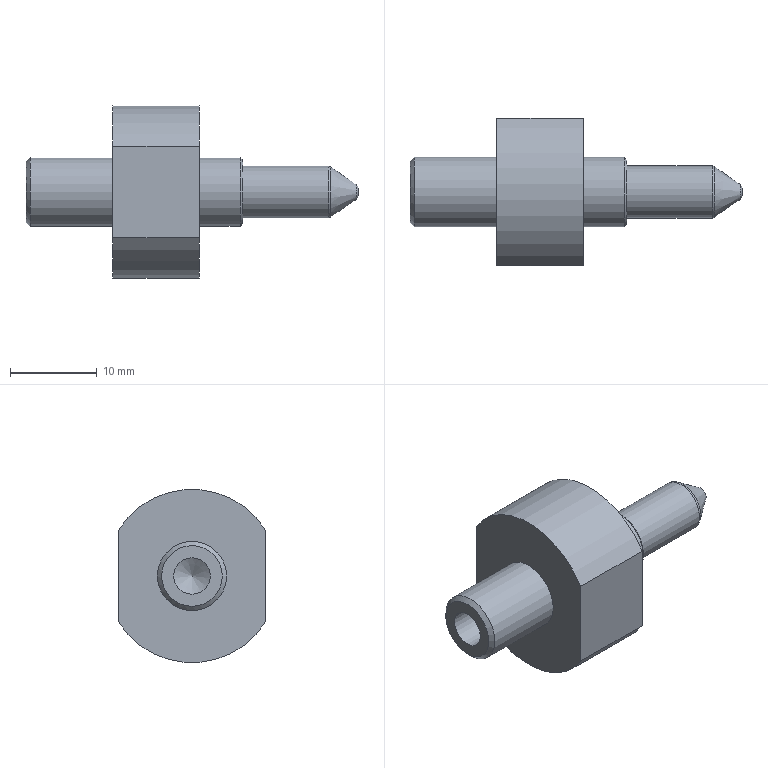Part | NX | features BREP 1 | 1 solid | 19 faces | box 38.285 x 17 x 20 mm | volume 3822 mm3 | plane 7 | cylinder 6 | cone 4 | torus 2 | commonest cylinder face diameters 8 x2 20 x2 4.2 x1 6 x1
STEP:
#1=CARTESIAN_POINT('',(-9.142,8.5,-5.268));
#2=VERTEX_POINT('',#1);
#3=CARTESIAN_POINT('',(-9.142,8.5,5.268));
#4=VERTEX_POINT('',#3);
#5=CARTESIAN_POINT('',(-9.142,8.5,0.));
#6=DIRECTION('',(0.,0.,1.));
#7=VECTOR('',#6,1000.);
#8=LINE('',#5,#7);
#9=EDGE_CURVE('',#2,#4,#8,.T.);
#10=ORIENTED_EDGE('',*,*,#9,.F.);
#11=CARTESIAN_POINT('',(-9.142,-8.5,-5.268));
#12=VERTEX_POINT('',#11);
#13=CARTESIAN_POINT('',(-9.142,0.,0.));
#14=DIRECTION('',(1.,0.,0.));
#15=DIRECTION('',(0.,-1.,0.));
#16=AXIS2_PLACEMENT_3D('',#13,#14,#15);
#17=CIRCLE('',#16,10.);
#18=EDGE_CURVE('',#12,#2,#17,.T.);
#19=ORIENTED_EDGE('',*,*,#18,.F.);
#20=CARTESIAN_POINT('',(-9.142,-8.5,5.268));
#21=VERTEX_POINT('',#20);
#22=CARTESIAN_POINT('',(-9.142,-8.5,0.));
#23=DIRECTION('',(0.,0.,-1.));
#24=VECTOR('',#23,1000.);
#25=LINE('',#22,#24);
#26=EDGE_CURVE('',#21,#12,#25,.T.);
#27=ORIENTED_EDGE('',*,*,#26,.F.);
#28=CARTESIAN_POINT('',(-9.142,0.,0.));
#29=DIRECTION('',(1.,0.,0.));
#30=DIRECTION('',(0.,-1.,0.));
#31=AXIS2_PLACEMENT_3D('',#28,#29,#30);
#32=CIRCLE('',#31,10.);
#33=EDGE_CURVE('',#4,#21,#32,.T.);
#34=ORIENTED_EDGE('',*,*,#33,.F.);
#35=EDGE_LOOP('',(#10,#19,#27,#34));
#36=FACE_BOUND('',#35,.T.);
#37=CARTESIAN_POINT('',(-9.142,-4.,0.));
#38=VERTEX_POINT('',#37);
#39=CARTESIAN_POINT('',(-9.142,0.,0.));
#40=DIRECTION('',(-1.,0.,0.));
#41=DIRECTION('',(0.,-1.,0.));
#42=AXIS2_PLACEMENT_3D('',#39,#40,#41);
#43=CIRCLE('',#42,4.);
#44=EDGE_CURVE('',#38,#38,#43,.T.);
#45=ORIENTED_EDGE('',*,*,#44,.F.);
#46=EDGE_LOOP('',(#45));
#47=FACE_BOUND('',#46,.T.);
#48=CARTESIAN_POINT('',(-9.142,10.,0.));
#49=DIRECTION('',(1.,0.,0.));
#50=DIRECTION('',(0.,-1.,0.));
#51=AXIS2_PLACEMENT_3D('',#48,#49,#50);
#52=PLANE('',#51);
#53=ADVANCED_FACE('',(#36,#47),#52,.F.);
#54=ORIENTED_EDGE('',*,*,#33,.T.);
#55=CARTESIAN_POINT('',(0.8576,-8.5,5.268));
#56=VERTEX_POINT('',#55);
#57=CARTESIAN_POINT('',(-19.142,-8.5,5.268));
#58=DIRECTION('',(1.,0.,0.));
#59=VECTOR('',#58,1000.);
#60=LINE('',#57,#59);
#61=EDGE_CURVE('',#21,#56,#60,.T.);
#62=ORIENTED_EDGE('',*,*,#61,.T.);
#63=CARTESIAN_POINT('',(0.8576,8.5,5.268));
#64=VERTEX_POINT('',#63);
#65=CARTESIAN_POINT('',(0.8576,0.,0.));
#66=DIRECTION('',(-1.,0.,0.));
#67=DIRECTION('',(0.,-1.,0.));
#68=AXIS2_PLACEMENT_3D('',#65,#66,#67);
#69=CIRCLE('',#68,10.);
#70=EDGE_CURVE('',#56,#64,#69,.T.);
#71=ORIENTED_EDGE('',*,*,#70,.T.);
#72=CARTESIAN_POINT('',(-19.142,8.5,5.268));
#73=DIRECTION('',(-1.,0.,0.));
#74=VECTOR('',#73,1000.);
#75=LINE('',#72,#74);
#76=EDGE_CURVE('',#64,#4,#75,.T.);
#77=ORIENTED_EDGE('',*,*,#76,.T.);
#78=EDGE_LOOP('',(#54,#62,#71,#77));
#79=FACE_BOUND('',#78,.T.);
#80=CARTESIAN_POINT('',(-19.142,0.,0.));
#81=DIRECTION('',(-1.,0.,0.));
#82=DIRECTION('',(0.,1.,0.));
#83=AXIS2_PLACEMENT_3D('',#80,#81,#82);
#84=CYLINDRICAL_SURFACE('',#83,10.);
#85=ADVANCED_FACE('',(#79),#84,.T.);
#86=CARTESIAN_POINT('',(0.8576,8.5,-5.268));
#87=VERTEX_POINT('',#86);
#88=CARTESIAN_POINT('',(19.142,8.5,-5.268));
#89=DIRECTION('',(1.,0.,0.));
#90=VECTOR('',#89,1000.);
#91=LINE('',#88,#90);
#92=EDGE_CURVE('',#2,#87,#91,.T.);
#93=ORIENTED_EDGE('',*,*,#92,.F.);
#94=ORIENTED_EDGE('',*,*,#9,.T.);
#95=ORIENTED_EDGE('',*,*,#76,.F.);
#96=CARTESIAN_POINT('',(0.8576,8.5,15.997));
#97=DIRECTION('',(0.,0.,1.));
#98=VECTOR('',#97,1000.);
#99=LINE('',#96,#98);
#100=EDGE_CURVE('',#87,#64,#99,.T.);
#101=ORIENTED_EDGE('',*,*,#100,.F.);
#102=EDGE_LOOP('',(#93,#94,#95,#101));
#103=FACE_BOUND('',#102,.T.);
#104=CARTESIAN_POINT('',(19.142,8.5,15.997));
#105=DIRECTION('',(0.,-1.,0.));
#106=DIRECTION('',(0.,0.,1.));
#107=AXIS2_PLACEMENT_3D('',#104,#105,#106);
#108=PLANE('',#107);
#109=ADVANCED_FACE('',(#103),#108,.F.);
#110=CARTESIAN_POINT('',(0.8576,-8.5,-5.268));
#111=VERTEX_POINT('',#110);
#112=CARTESIAN_POINT('',(0.8576,0.,0.));
#113=DIRECTION('',(-1.,0.,0.));
#114=DIRECTION('',(0.,-1.,0.));
#115=AXIS2_PLACEMENT_3D('',#112,#113,#114);
#116=CIRCLE('',#115,10.);
#117=EDGE_CURVE('',#87,#111,#116,.T.);
#118=ORIENTED_EDGE('',*,*,#117,.T.);
#119=CARTESIAN_POINT('',(-19.142,-8.5,-5.268));
#120=DIRECTION('',(-1.,0.,0.));
#121=VECTOR('',#120,1000.);
#122=LINE('',#119,#121);
#123=EDGE_CURVE('',#111,#12,#122,.T.);
#124=ORIENTED_EDGE('',*,*,#123,.T.);
#125=ORIENTED_EDGE('',*,*,#18,.T.);
#126=ORIENTED_EDGE('',*,*,#92,.T.);
#127=EDGE_LOOP('',(#118,#124,#125,#126));
#128=FACE_BOUND('',#127,.T.);
#129=CARTESIAN_POINT('',(-19.142,0.,0.));
#130=DIRECTION('',(-1.,0.,0.));
#131=DIRECTION('',(0.,1.,0.));
#132=AXIS2_PLACEMENT_3D('',#129,#130,#131);
#133=CYLINDRICAL_SURFACE('',#132,10.);
#134=ADVANCED_FACE('',(#128),#133,.T.);
#135=ORIENTED_EDGE('',*,*,#61,.F.);
#136=ORIENTED_EDGE('',*,*,#26,.T.);
#137=ORIENTED_EDGE('',*,*,#123,.F.);
#138=CARTESIAN_POINT('',(0.8576,-8.5,13.741));
#139=DIRECTION('',(0.,0.,-1.));
#140=VECTOR('',#139,1000.);
#141=LINE('',#138,#140);
#142=EDGE_CURVE('',#56,#111,#141,.T.);
#143=ORIENTED_EDGE('',*,*,#142,.F.);
#144=EDGE_LOOP('',(#135,#136,#137,#143));
#145=FACE_BOUND('',#144,.T.);
#146=CARTESIAN_POINT('',(19.142,-8.5,13.741));
#147=DIRECTION('',(0.,1.,0.));
#148=DIRECTION('',(0.,0.,-1.));
#149=AXIS2_PLACEMENT_3D('',#146,#147,#148);
#150=PLANE('',#149);
#151=ADVANCED_FACE('',(#145),#150,.F.);
#152=CARTESIAN_POINT('',(-18.642,-4.,0.));
#153=VERTEX_POINT('',#152);
#154=CARTESIAN_POINT('',(-18.642,0.,0.));
#155=DIRECTION('',(1.,0.,0.));
#156=DIRECTION('',(0.,-1.,0.));
#157=AXIS2_PLACEMENT_3D('',#154,#155,#156);
#158=CIRCLE('',#157,4.);
#159=EDGE_CURVE('',#153,#153,#158,.T.);
#160=ORIENTED_EDGE('',*,*,#159,.T.);
#161=EDGE_LOOP('',(#160));
#162=FACE_BOUND('',#161,.T.);
#163=ORIENTED_EDGE('',*,*,#44,.T.);
#164=EDGE_LOOP('',(#163));
#165=FACE_BOUND('',#164,.T.);
#166=CARTESIAN_POINT('',(-19.142,0.,0.));
#167=DIRECTION('',(-1.,0.,0.));
#168=DIRECTION('',(0.,1.,0.));
#169=AXIS2_PLACEMENT_3D('',#166,#167,#168);
#170=CYLINDRICAL_SURFACE('',#169,4.);
#171=ADVANCED_FACE('',(#162,#165),#170,.T.);
#172=CARTESIAN_POINT('',(0.8576,-4.,0.));
#173=VERTEX_POINT('',#172);
#174=CARTESIAN_POINT('',(0.8576,0.,0.));
#175=DIRECTION('',(1.,0.,0.));
#176=DIRECTION('',(0.,-1.,0.));
#177=AXIS2_PLACEMENT_3D('',#174,#175,#176);
#178=CIRCLE('',#177,4.);
#179=EDGE_CURVE('',#173,#173,#178,.T.);
#180=ORIENTED_EDGE('',*,*,#179,.F.);
#181=EDGE_LOOP('',(#180));
#182=FACE_BOUND('',#181,.T.);
#183=ORIENTED_EDGE('',*,*,#100,.T.);
#184=ORIENTED_EDGE('',*,*,#70,.F.);
#185=ORIENTED_EDGE('',*,*,#142,.T.);
#186=ORIENTED_EDGE('',*,*,#117,.F.);
#187=EDGE_LOOP('',(#183,#184,#185,#186));
#188=FACE_BOUND('',#187,.T.);
#189=CARTESIAN_POINT('',(0.8576,4.,0.));
#190=DIRECTION('',(-1.,0.,0.));
#191=DIRECTION('',(0.,1.,0.));
#192=AXIS2_PLACEMENT_3D('',#189,#190,#191);
#193=PLANE('',#192);
#194=ADVANCED_FACE('',(#182,#188),#193,.F.);
#195=ORIENTED_EDGE('',*,*,#159,.F.);
#196=EDGE_LOOP('',(#195));
#197=FACE_BOUND('',#196,.T.);
#198=CARTESIAN_POINT('',(-19.142,0.,-3.5));
#199=VERTEX_POINT('',#198);
#200=CARTESIAN_POINT('',(-19.142,0.,0.));
#201=DIRECTION('',(1.,0.,0.));
#202=DIRECTION('',(0.,0.,-1.));
#203=AXIS2_PLACEMENT_3D('',#200,#201,#202);
#204=CIRCLE('',#203,3.5);
#205=EDGE_CURVE('',#199,#199,#204,.T.);
#206=ORIENTED_EDGE('',*,*,#205,.T.);
#207=EDGE_LOOP('',(#206));
#208=FACE_BOUND('',#207,.T.);
#209=CARTESIAN_POINT('',(-18.642,0.,0.));
#210=DIRECTION('',(1.,0.,0.));
#211=DIRECTION('',(0.,0.,1.));
#212=AXIS2_PLACEMENT_3D('',#209,#210,#211);
#213=CONICAL_SURFACE('',#212,4.,0.7854);
#214=ADVANCED_FACE('',(#197,#208),#213,.T.);
#215=ORIENTED_EDGE('',*,*,#179,.T.);
#216=EDGE_LOOP('',(#215));
#217=FACE_BOUND('',#216,.T.);
#218=CARTESIAN_POINT('',(5.558,-4.,0.));
#219=VERTEX_POINT('',#218);
#220=CARTESIAN_POINT('',(5.558,0.,0.));
#221=DIRECTION('',(-1.,0.,0.));
#222=DIRECTION('',(0.,-1.,0.));
#223=AXIS2_PLACEMENT_3D('',#220,#221,#222);
#224=CIRCLE('',#223,4.);
#225=EDGE_CURVE('',#219,#219,#224,.T.);
#226=ORIENTED_EDGE('',*,*,#225,.T.);
#227=EDGE_LOOP('',(#226));
#228=FACE_BOUND('',#227,.T.);
#229=CARTESIAN_POINT('',(-19.142,0.,0.));
#230=DIRECTION('',(-1.,0.,0.));
#231=DIRECTION('',(0.,1.,0.));
#232=AXIS2_PLACEMENT_3D('',#229,#230,#231);
#233=CYLINDRICAL_SURFACE('',#232,4.);
#234=ADVANCED_FACE('',(#217,#228),#233,.T.);
#235=CARTESIAN_POINT('',(-19.142,0.,2.1));
#236=VERTEX_POINT('',#235);
#237=CARTESIAN_POINT('',(-19.142,0.,0.));
#238=DIRECTION('',(-1.,0.,0.));
#239=DIRECTION('',(0.,0.,1.));
#240=AXIS2_PLACEMENT_3D('',#237,#238,#239);
#241=CIRCLE('',#240,2.1);
#242=EDGE_CURVE('',#236,#236,#241,.T.);
#243=ORIENTED_EDGE('',*,*,#242,.F.);
#244=EDGE_LOOP('',(#243));
#245=FACE_BOUND('',#244,.T.);
#246=ORIENTED_EDGE('',*,*,#205,.F.);
#247=EDGE_LOOP('',(#246));
#248=FACE_BOUND('',#247,.T.);
#249=CARTESIAN_POINT('',(-19.142,4.,0.));
#250=DIRECTION('',(1.,0.,0.));
#251=DIRECTION('',(0.,-1.,0.));
#252=AXIS2_PLACEMENT_3D('',#249,#250,#251);
#253=PLANE('',#252);
#254=ADVANCED_FACE('',(#245,#248),#253,.F.);
#255=ORIENTED_EDGE('',*,*,#225,.F.);
#256=EDGE_LOOP('',(#255));
#257=FACE_BOUND('',#256,.T.);
#258=CARTESIAN_POINT('',(5.858,0.,3.7));
#259=VERTEX_POINT('',#258);
#260=CARTESIAN_POINT('',(5.858,0.,0.));
#261=DIRECTION('',(-1.,0.,0.));
#262=DIRECTION('',(0.,0.,1.));
#263=AXIS2_PLACEMENT_3D('',#260,#261,#262);
#264=CIRCLE('',#263,3.7);
#265=EDGE_CURVE('',#259,#259,#264,.T.);
#266=ORIENTED_EDGE('',*,*,#265,.T.);
#267=EDGE_LOOP('',(#266));
#268=FACE_BOUND('',#267,.T.);
#269=CARTESIAN_POINT('',(5.558,0.,0.));
#270=DIRECTION('',(-1.,0.,0.));
#271=DIRECTION('',(0.,0.,-1.));
#272=AXIS2_PLACEMENT_3D('',#269,#270,#271);
#273=CONICAL_SURFACE('',#272,4.,0.7854);
#274=ADVANCED_FACE('',(#257,#268),#273,.T.);
#275=CARTESIAN_POINT('',(-6.742,0.,2.1));
#276=VERTEX_POINT('',#275);
#277=CARTESIAN_POINT('',(-6.742,0.,0.));
#278=DIRECTION('',(-1.,0.,0.));
#279=DIRECTION('',(0.,0.,1.));
#280=AXIS2_PLACEMENT_3D('',#277,#278,#279);
#281=CIRCLE('',#280,2.1);
#282=EDGE_CURVE('',#276,#276,#281,.T.);
#283=ORIENTED_EDGE('',*,*,#282,.F.);
#284=EDGE_LOOP('',(#283));
#285=FACE_BOUND('',#284,.T.);
#286=ORIENTED_EDGE('',*,*,#242,.T.);
#287=EDGE_LOOP('',(#286));
#288=FACE_BOUND('',#287,.T.);
#289=CARTESIAN_POINT('',(-19.142,0.,0.));
#290=DIRECTION('',(-1.,0.,0.));
#291=DIRECTION('',(0.,0.,-1.));
#292=AXIS2_PLACEMENT_3D('',#289,#290,#291);
#293=CYLINDRICAL_SURFACE('',#292,2.1);
#294=ADVANCED_FACE('',(#285,#288),#293,.F.);
#295=CARTESIAN_POINT('',(5.858,-3.,0.));
#296=VERTEX_POINT('',#295);
#297=CARTESIAN_POINT('',(5.858,0.,0.));
#298=DIRECTION('',(1.,0.,0.));
#299=DIRECTION('',(0.,-1.,0.));
#300=AXIS2_PLACEMENT_3D('',#297,#298,#299);
#301=CIRCLE('',#300,3.);
#302=EDGE_CURVE('',#296,#296,#301,.T.);
#303=ORIENTED_EDGE('',*,*,#302,.F.);
#304=EDGE_LOOP('',(#303));
#305=FACE_BOUND('',#304,.T.);
#306=ORIENTED_EDGE('',*,*,#265,.F.);
#307=EDGE_LOOP('',(#306));
#308=FACE_BOUND('',#307,.T.);
#309=CARTESIAN_POINT('',(5.858,3.,0.));
#310=DIRECTION('',(-1.,0.,0.));
#311=DIRECTION('',(0.,1.,0.));
#312=AXIS2_PLACEMENT_3D('',#309,#310,#311);
#313=PLANE('',#312);
#314=ADVANCED_FACE('',(#305,#308),#313,.F.);
#315=CARTESIAN_POINT('',(-5.481,0.,0.));
#316=VERTEX_POINT('',#315);
#317=VERTEX_LOOP('',#316);
#318=FACE_BOUND('',#317,.T.);
#319=ORIENTED_EDGE('',*,*,#282,.T.);
#320=EDGE_LOOP('',(#319));
#321=FACE_BOUND('',#320,.T.);
#322=CARTESIAN_POINT('',(-6.742,0.,0.));
#323=DIRECTION('',(-1.,0.,0.));
#324=DIRECTION('',(0.,0.,-1.));
#325=AXIS2_PLACEMENT_3D('',#322,#323,#324);
#326=CONICAL_SURFACE('',#325,2.1,1.03);
#327=ADVANCED_FACE('',(#318,#321),#326,.F.);
#328=ORIENTED_EDGE('',*,*,#302,.T.);
#329=EDGE_LOOP('',(#328));
#330=FACE_BOUND('',#329,.T.);
#331=CARTESIAN_POINT('',(15.7,-3.,0.));
#332=VERTEX_POINT('',#331);
#333=CARTESIAN_POINT('',(15.7,0.,0.));
#334=DIRECTION('',(-1.,0.,0.));
#335=DIRECTION('',(0.,-1.,0.));
#336=AXIS2_PLACEMENT_3D('',#333,#334,#335);
#337=CIRCLE('',#336,3.);
#338=EDGE_CURVE('',#332,#332,#337,.T.);
#339=ORIENTED_EDGE('',*,*,#338,.T.);
#340=EDGE_LOOP('',(#339));
#341=FACE_BOUND('',#340,.T.);
#342=CARTESIAN_POINT('',(-19.142,0.,0.));
#343=DIRECTION('',(-1.,0.,0.));
#344=DIRECTION('',(0.,1.,0.));
#345=AXIS2_PLACEMENT_3D('',#342,#343,#344);
#346=CYLINDRICAL_SURFACE('',#345,3.);
#347=ADVANCED_FACE('',(#330,#341),#346,.T.);
#348=CARTESIAN_POINT('',(15.987,2.91,0.));
#349=VERTEX_POINT('',#348);
#350=CARTESIAN_POINT('',(15.987,0.,0.));
#351=DIRECTION('',(-1.,0.,0.));
#352=DIRECTION('',(0.,1.,0.));
#353=AXIS2_PLACEMENT_3D('',#350,#351,#352);
#354=CIRCLE('',#353,2.91);
#355=EDGE_CURVE('',#349,#349,#354,.T.);
#356=ORIENTED_EDGE('',*,*,#355,.T.);
#357=EDGE_LOOP('',(#356));
#358=FACE_BOUND('',#357,.T.);
#359=ORIENTED_EDGE('',*,*,#338,.F.);
#360=EDGE_LOOP('',(#359));
#361=FACE_BOUND('',#360,.T.);
#362=CARTESIAN_POINT('',(15.7,0.,0.));
#363=DIRECTION('',(1.,0.,0.));
#364=DIRECTION('',(0.,0.,-1.));
#365=AXIS2_PLACEMENT_3D('',#362,#363,#364);
#366=TOROIDAL_SURFACE('',#365,2.5,0.5);
#367=ADVANCED_FACE('',(#358,#361),#366,.T.);
#368=ORIENTED_EDGE('',*,*,#355,.F.);
#369=EDGE_LOOP('',(#368));
#370=FACE_BOUND('',#369,.T.);
#371=CARTESIAN_POINT('',(18.929,-0.8493,0.));
#372=VERTEX_POINT('',#371);
#373=CARTESIAN_POINT('',(18.929,0.,0.));
#374=DIRECTION('',(-1.,0.,0.));
#375=DIRECTION('',(0.,-1.,0.));
#376=AXIS2_PLACEMENT_3D('',#373,#374,#375);
#377=CIRCLE('',#376,0.8493);
#378=EDGE_CURVE('',#372,#372,#377,.T.);
#379=ORIENTED_EDGE('',*,*,#378,.T.);
#380=EDGE_LOOP('',(#379));
#381=FACE_BOUND('',#380,.T.);
#382=CARTESIAN_POINT('',(15.987,0.,0.));
#383=DIRECTION('',(-1.,0.,0.));
#384=DIRECTION('',(0.,0.,-1.));
#385=AXIS2_PLACEMENT_3D('',#382,#383,#384);
#386=CONICAL_SURFACE('',#385,2.91,0.6109);
#387=ADVANCED_FACE('',(#370,#381),#386,.T.);
#388=ORIENTED_EDGE('',*,*,#378,.F.);
#389=EDGE_LOOP('',(#388));
#390=FACE_BOUND('',#389,.T.);
#391=CARTESIAN_POINT('',(19.142,-0.4397,0.));
#392=VERTEX_POINT('',#391);
#393=CARTESIAN_POINT('',(19.142,0.4397,0.));
#394=VERTEX_POINT('',#393);
#395=CARTESIAN_POINT('',(19.142,0.,0.));
#396=DIRECTION('',(-1.,0.,0.));
#397=DIRECTION('',(0.,0.,1.));
#398=AXIS2_PLACEMENT_3D('',#395,#396,#397);
#399=CIRCLE('',#398,0.4397);
#400=EDGE_CURVE('',#392,#394,#399,.T.);
#401=ORIENTED_EDGE('',*,*,#400,.T.);
#402=CARTESIAN_POINT('',(19.142,0.,0.));
#403=DIRECTION('',(-1.,0.,0.));
#404=DIRECTION('',(0.,0.,1.));
#405=AXIS2_PLACEMENT_3D('',#402,#403,#404);
#406=CIRCLE('',#405,0.4397);
#407=EDGE_CURVE('',#394,#392,#406,.T.);
#408=ORIENTED_EDGE('',*,*,#407,.T.);
#409=EDGE_LOOP('',(#401,#408));
#410=FACE_BOUND('',#409,.T.);
#411=CARTESIAN_POINT('',(18.642,0.,0.));
#412=DIRECTION('',(-1.,0.,0.));
#413=DIRECTION('',(0.,0.,1.));
#414=AXIS2_PLACEMENT_3D('',#411,#412,#413);
#415=DEGENERATE_TOROIDAL_SURFACE('',#414,0.4397,0.5,.T.);
#416=ADVANCED_FACE('',(#390,#410),#415,.T.);
#417=ORIENTED_EDGE('',*,*,#400,.F.);
#418=ORIENTED_EDGE('',*,*,#407,.F.);
#419=EDGE_LOOP('',(#417,#418));
#420=FACE_BOUND('',#419,.T.);
#421=CARTESIAN_POINT('',(19.142,0.,0.));
#422=DIRECTION('',(-1.,0.,0.));
#423=DIRECTION('',(0.,1.,0.));
#424=AXIS2_PLACEMENT_3D('',#421,#422,#423);
#425=PLANE('',#424);
#426=ADVANCED_FACE('',(#420),#425,.F.);
#427=CLOSED_SHELL('',(#53,#85,#109,#134,#151,#171,#194,#214,#234,#254,#274,#294,#314,#327,#347,#367,#387,#416,#426));
#428=MANIFOLD_SOLID_BREP('',#427);
#429=(LENGTH_UNIT()NAMED_UNIT(*)SI_UNIT(.MILLI.,.METRE.));
#430=UNCERTAINTY_MEASURE_WITH_UNIT(LENGTH_MEASURE(0.00001),#429,'','');
#431=(NAMED_UNIT(*)PLANE_ANGLE_UNIT()SI_UNIT($,.RADIAN.));
#432=(NAMED_UNIT(*)SI_UNIT($,.STERADIAN.)SOLID_ANGLE_UNIT());
#433=(GEOMETRIC_REPRESENTATION_CONTEXT(3)GLOBAL_UNCERTAINTY_ASSIGNED_CONTEXT((#430))GLOBAL_UNIT_ASSIGNED_CONTEXT((#429,#431,#432))REPRESENTATION_CONTEXT('',''));
#434=ADVANCED_BREP_SHAPE_REPRESENTATION('',(#428),#433);